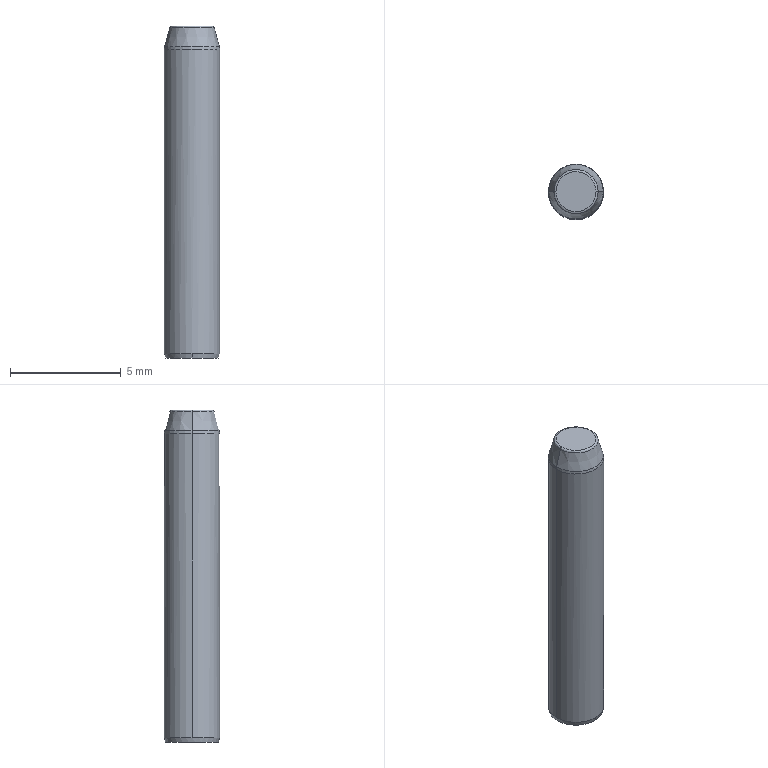Part | SolidWorks | features BaseBody 1 | 1 solid | 12 faces | box 2.5 x 2.5 x 15 mm | volume 72.605 mm3 | spline 4 | cone 4 | cylinder 2 | plane 2 | commonest cylinder face diameters 2.5 x2
STEP:
#1=CARTESIAN_POINT('',(1.233,0.,14.064));
#2=VERTEX_POINT('',#1);
#3=CARTESIAN_POINT('',(-1.233,0.,14.064));
#4=VERTEX_POINT('',#3);
#5=CARTESIAN_POINT('',(0.,0.,14.064));
#6=DIRECTION('',(0.,0.,-1.));
#7=DIRECTION('',(1.,0.,0.));
#8=AXIS2_PLACEMENT_3D('',#5,#6,#7);
#9=CIRCLE('',#8,1.233);
#10=EDGE_CURVE('',#2,#4,#9,.T.);
#11=ORIENTED_EDGE('',*,*,#10,.T.);
#12=CARTESIAN_POINT('',(-1.25,0.,13.934));
#13=VERTEX_POINT('',#12);
#14=CARTESIAN_POINT('',(-0.75,0.,13.934));
#15=DIRECTION('',(0.,-1.,0.));
#16=DIRECTION('',(-1.,0.,0.));
#17=AXIS2_PLACEMENT_3D('',#14,#15,#16);
#18=CIRCLE('',#17,0.5);
#19=EDGE_CURVE('',#4,#13,#18,.T.);
#20=ORIENTED_EDGE('',*,*,#19,.T.);
#21=CARTESIAN_POINT('',(1.25,0.,13.934));
#22=VERTEX_POINT('',#21);
#23=CARTESIAN_POINT('',(0.,0.,13.934));
#24=DIRECTION('',(0.,0.,-1.));
#25=DIRECTION('',(1.,0.,0.));
#26=AXIS2_PLACEMENT_3D('',#23,#24,#25);
#27=CIRCLE('',#26,1.25);
#28=EDGE_CURVE('',#22,#13,#27,.T.);
#29=ORIENTED_EDGE('',*,*,#28,.F.);
#30=CARTESIAN_POINT('',(0.75,0.,13.934));
#31=DIRECTION('',(0.,1.,0.));
#32=DIRECTION('',(1.,0.,0.));
#33=AXIS2_PLACEMENT_3D('',#30,#31,#32);
#34=CIRCLE('',#33,0.5);
#35=EDGE_CURVE('',#2,#22,#34,.T.);
#36=ORIENTED_EDGE('',*,*,#35,.F.);
#37=EDGE_LOOP('',(#11,#20,#29,#36));
#38=FACE_OUTER_BOUND('',#37,.T.);
#39=CARTESIAN_POINT('',(-1.233,0.,14.064));
#40=CARTESIAN_POINT('',(-1.233,-2.466,14.064));
#41=CARTESIAN_POINT('',(1.233,-2.466,14.064));
#42=CARTESIAN_POINT('',(1.233,0.,14.064));
#43=CARTESIAN_POINT('',(-1.244,0.,14.021));
#44=CARTESIAN_POINT('',(-1.244,-2.489,14.021));
#45=CARTESIAN_POINT('',(1.244,-2.489,14.021));
#46=CARTESIAN_POINT('',(1.244,0.,14.021));
#47=CARTESIAN_POINT('',(-1.25,0.,13.978));
#48=CARTESIAN_POINT('',(-1.25,-2.5,13.978));
#49=CARTESIAN_POINT('',(1.25,-2.5,13.978));
#50=CARTESIAN_POINT('',(1.25,0.,13.978));
#51=CARTESIAN_POINT('',(-1.25,0.,13.934));
#52=CARTESIAN_POINT('',(-1.25,-2.5,13.934));
#53=CARTESIAN_POINT('',(1.25,-2.5,13.934));
#54=CARTESIAN_POINT('',(1.25,0.,13.934));
#55=(BOUNDED_SURFACE()B_SPLINE_SURFACE(3,3,((#39,#40,#41,#42),(#43,#44,#45,#46),(#47,#48,#49,#50),(#51,#52,#53,#54)),.UNSPECIFIED.,.F.,.F.,.T.)B_SPLINE_SURFACE_WITH_KNOTS((4,4),(4,4),(0.,1.),(0.,1.),.UNSPECIFIED.)GEOMETRIC_REPRESENTATION_ITEM()RATIONAL_B_SPLINE_SURFACE(((1.,0.3333,0.3333,1.),(0.9943,0.3314,0.3314,0.9943),(0.9943,0.3314,0.3314,0.9943),(1.,0.3333,0.3333,1.)))REPRESENTATION_ITEM('')SURFACE());
#56=ADVANCED_FACE('',(#38),#55,.T.);
#57=CARTESIAN_POINT('',(1.002,0.,14.926));
#58=VERTEX_POINT('',#57);
#59=CARTESIAN_POINT('',(-1.002,0.,14.926));
#60=VERTEX_POINT('',#59);
#61=CARTESIAN_POINT('',(0.,0.,14.926));
#62=DIRECTION('',(0.,0.,-1.));
#63=DIRECTION('',(-1.,0.,0.));
#64=AXIS2_PLACEMENT_3D('',#61,#62,#63);
#65=CIRCLE('',#64,1.002);
#66=EDGE_CURVE('',#58,#60,#65,.T.);
#67=ORIENTED_EDGE('',*,*,#66,.F.);
#68=CARTESIAN_POINT('',(0.9053,0.,15.));
#69=VERTEX_POINT('',#68);
#70=CARTESIAN_POINT('',(0.9053,0.,14.9));
#71=DIRECTION('',(0.,-1.,0.));
#72=DIRECTION('',(1.,0.,0.));
#73=AXIS2_PLACEMENT_3D('',#70,#71,#72);
#74=CIRCLE('',#73,0.1);
#75=EDGE_CURVE('',#58,#69,#74,.T.);
#76=ORIENTED_EDGE('',*,*,#75,.T.);
#77=CARTESIAN_POINT('',(-0.9053,0.,15.));
#78=VERTEX_POINT('',#77);
#79=CARTESIAN_POINT('',(0.9053,0.,15.));
#80=CARTESIAN_POINT('',(0.9053,-1.811,15.));
#81=CARTESIAN_POINT('',(-0.9053,-1.811,15.));
#82=CARTESIAN_POINT('',(-0.9053,0.,15.));
#83=(BOUNDED_CURVE()B_SPLINE_CURVE(3,(#79,#80,#81,#82),.UNSPECIFIED.,.F.,.F.)B_SPLINE_CURVE_WITH_KNOTS((4,4),(0.,0.5),.UNSPECIFIED.)CURVE()GEOMETRIC_REPRESENTATION_ITEM()RATIONAL_B_SPLINE_CURVE((1.,0.3333,0.3333,1.))REPRESENTATION_ITEM(''));
#84=EDGE_CURVE('',#69,#78,#83,.T.);
#85=ORIENTED_EDGE('',*,*,#84,.T.);
#86=CARTESIAN_POINT('',(-0.9053,0.,14.9));
#87=DIRECTION('',(0.,1.,0.));
#88=DIRECTION('',(-1.,0.,0.));
#89=AXIS2_PLACEMENT_3D('',#86,#87,#88);
#90=CIRCLE('',#89,0.1);
#91=EDGE_CURVE('',#60,#78,#90,.T.);
#92=ORIENTED_EDGE('',*,*,#91,.F.);
#93=EDGE_LOOP('',(#67,#76,#85,#92));
#94=FACE_OUTER_BOUND('',#93,.T.);
#95=CARTESIAN_POINT('',(1.002,0.,14.926));
#96=CARTESIAN_POINT('',(1.002,-2.004,14.926));
#97=CARTESIAN_POINT('',(-1.002,-2.004,14.926));
#98=CARTESIAN_POINT('',(-1.002,0.,14.926));
#99=CARTESIAN_POINT('',(0.9897,0.,14.971));
#100=CARTESIAN_POINT('',(0.9897,-1.979,14.971));
#101=CARTESIAN_POINT('',(-0.9897,-1.979,14.971));
#102=CARTESIAN_POINT('',(-0.9897,0.,14.971));
#103=CARTESIAN_POINT('',(0.9524,0.,15.));
#104=CARTESIAN_POINT('',(0.9524,-1.905,15.));
#105=CARTESIAN_POINT('',(-0.9524,-1.905,15.));
#106=CARTESIAN_POINT('',(-0.9524,0.,15.));
#107=CARTESIAN_POINT('',(0.9053,0.,15.));
#108=CARTESIAN_POINT('',(0.9053,-1.811,15.));
#109=CARTESIAN_POINT('',(-0.9053,-1.811,15.));
#110=CARTESIAN_POINT('',(-0.9053,0.,15.));
#111=(BOUNDED_SURFACE()B_SPLINE_SURFACE(3,3,((#95,#96,#97,#98),(#99,#100,#101,#102),(#103,#104,#105,#106),(#107,#108,#109,#110)),.UNSPECIFIED.,.F.,.F.,.T.)B_SPLINE_SURFACE_WITH_KNOTS((4,4),(4,4),(0.,1.),(0.,1.),.UNSPECIFIED.)GEOMETRIC_REPRESENTATION_ITEM()RATIONAL_B_SPLINE_SURFACE(((1.,0.3333,0.3333,1.),(0.8622,0.2874,0.2874,0.8622),(0.8622,0.2874,0.2874,0.8622),(1.,0.3333,0.3333,1.)))REPRESENTATION_ITEM('')SURFACE());
#112=ADVANCED_FACE('',(#94),#111,.T.);
#113=CARTESIAN_POINT('',(0.,1.25,0.2));
#114=VERTEX_POINT('',#113);
#115=CARTESIAN_POINT('',(-1.25,0.,0.2));
#116=VERTEX_POINT('',#115);
#117=CARTESIAN_POINT('',(0.,0.,0.2));
#118=DIRECTION('',(0.,0.,1.));
#119=DIRECTION('',(1.,0.,0.));
#120=AXIS2_PLACEMENT_3D('',#117,#118,#119);
#121=CIRCLE('',#120,1.25);
#122=EDGE_CURVE('',#114,#116,#121,.T.);
#123=ORIENTED_EDGE('',*,*,#122,.T.);
#124=CARTESIAN_POINT('',(-1.25,0.,0.));
#125=DIRECTION('',(0.,0.,1.));
#126=VECTOR('',#125,1000.);
#127=LINE('',#124,#126);
#128=EDGE_CURVE('',#116,#13,#127,.T.);
#129=ORIENTED_EDGE('',*,*,#128,.T.);
#130=CARTESIAN_POINT('',(0.,0.,13.934));
#131=DIRECTION('',(0.,0.,-1.));
#132=DIRECTION('',(1.,0.,0.));
#133=AXIS2_PLACEMENT_3D('',#130,#131,#132);
#134=CIRCLE('',#133,1.25);
#135=EDGE_CURVE('',#13,#22,#134,.T.);
#136=ORIENTED_EDGE('',*,*,#135,.T.);
#137=CARTESIAN_POINT('',(1.25,0.,0.2));
#138=VERTEX_POINT('',#137);
#139=CARTESIAN_POINT('',(1.25,0.,0.));
#140=DIRECTION('',(0.,0.,1.));
#141=VECTOR('',#140,1000.);
#142=LINE('',#139,#141);
#143=EDGE_CURVE('',#138,#22,#142,.T.);
#144=ORIENTED_EDGE('',*,*,#143,.F.);
#145=CARTESIAN_POINT('',(0.,0.,0.2));
#146=DIRECTION('',(0.,0.,1.));
#147=DIRECTION('',(1.,0.,0.));
#148=AXIS2_PLACEMENT_3D('',#145,#146,#147);
#149=CIRCLE('',#148,1.25);
#150=EDGE_CURVE('',#138,#114,#149,.T.);
#151=ORIENTED_EDGE('',*,*,#150,.T.);
#152=EDGE_LOOP('',(#123,#129,#136,#144,#151));
#153=FACE_OUTER_BOUND('',#152,.T.);
#154=CARTESIAN_POINT('',(0.,0.,0.));
#155=DIRECTION('',(0.,0.,1.));
#156=DIRECTION('',(1.,0.,0.));
#157=AXIS2_PLACEMENT_3D('',#154,#155,#156);
#158=CYLINDRICAL_SURFACE('',#157,1.25);
#159=ADVANCED_FACE('',(#153),#158,.T.);
#160=CARTESIAN_POINT('',(0.,-1.196,0.));
#161=VERTEX_POINT('',#160);
#162=CARTESIAN_POINT('',(0.,1.196,0.));
#163=VERTEX_POINT('',#162);
#164=CARTESIAN_POINT('',(0.,0.,0.));
#165=DIRECTION('',(0.,0.,1.));
#166=DIRECTION('',(0.,-1.,0.));
#167=AXIS2_PLACEMENT_3D('',#164,#165,#166);
#168=CIRCLE('',#167,1.196);
#169=EDGE_CURVE('',#161,#163,#168,.T.);
#170=ORIENTED_EDGE('',*,*,#169,.T.);
#171=CARTESIAN_POINT('',(0.,1.25,0.2));
#172=DIRECTION('',(0.,0.2588,0.9659));
#173=VECTOR('',#172,1000.);
#174=LINE('',#171,#173);
#175=EDGE_CURVE('',#163,#114,#174,.T.);
#176=ORIENTED_EDGE('',*,*,#175,.T.);
#177=ORIENTED_EDGE('',*,*,#150,.F.);
#178=CARTESIAN_POINT('',(0.,-1.25,0.2));
#179=VERTEX_POINT('',#178);
#180=CARTESIAN_POINT('',(0.,0.,0.2));
#181=DIRECTION('',(0.,0.,1.));
#182=DIRECTION('',(1.,0.,0.));
#183=AXIS2_PLACEMENT_3D('',#180,#181,#182);
#184=CIRCLE('',#183,1.25);
#185=EDGE_CURVE('',#179,#138,#184,.T.);
#186=ORIENTED_EDGE('',*,*,#185,.F.);
#187=CARTESIAN_POINT('',(0.,-1.25,0.2));
#188=DIRECTION('',(0.,-0.2588,0.9659));
#189=VECTOR('',#188,1000.);
#190=LINE('',#187,#189);
#191=EDGE_CURVE('',#161,#179,#190,.T.);
#192=ORIENTED_EDGE('',*,*,#191,.F.);
#193=EDGE_LOOP('',(#170,#176,#177,#186,#192));
#194=FACE_OUTER_BOUND('',#193,.T.);
#195=CARTESIAN_POINT('',(0.,0.,0.2));
#196=DIRECTION('',(0.,0.,1.));
#197=DIRECTION('',(0.,-1.,0.));
#198=AXIS2_PLACEMENT_3D('',#195,#196,#197);
#199=CONICAL_SURFACE('',#198,1.25,0.2618);
#200=ADVANCED_FACE('',(#194),#199,.T.);
#201=CARTESIAN_POINT('',(0.,0.,14.926));
#202=DIRECTION('',(0.,0.,-1.));
#203=DIRECTION('',(-1.,0.,0.));
#204=AXIS2_PLACEMENT_3D('',#201,#202,#203);
#205=CIRCLE('',#204,1.002);
#206=EDGE_CURVE('',#60,#58,#205,.T.);
#207=ORIENTED_EDGE('',*,*,#206,.T.);
#208=CARTESIAN_POINT('',(1.233,0.,14.064));
#209=DIRECTION('',(0.2588,0.,-0.9659));
#210=VECTOR('',#209,1000.);
#211=LINE('',#208,#210);
#212=EDGE_CURVE('',#58,#2,#211,.T.);
#213=ORIENTED_EDGE('',*,*,#212,.T.);
#214=CARTESIAN_POINT('',(0.,0.,14.064));
#215=DIRECTION('',(0.,0.,-1.));
#216=DIRECTION('',(1.,0.,0.));
#217=AXIS2_PLACEMENT_3D('',#214,#215,#216);
#218=CIRCLE('',#217,1.233);
#219=EDGE_CURVE('',#4,#2,#218,.T.);
#220=ORIENTED_EDGE('',*,*,#219,.F.);
#221=CARTESIAN_POINT('',(-1.233,0.,14.064));
#222=DIRECTION('',(-0.2588,0.,-0.9659));
#223=VECTOR('',#222,1000.);
#224=LINE('',#221,#223);
#225=EDGE_CURVE('',#60,#4,#224,.T.);
#226=ORIENTED_EDGE('',*,*,#225,.F.);
#227=EDGE_LOOP('',(#207,#213,#220,#226));
#228=FACE_OUTER_BOUND('',#227,.T.);
#229=CARTESIAN_POINT('',(0.,0.,14.064));
#230=DIRECTION('',(0.,0.,-1.));
#231=DIRECTION('',(-1.,0.,0.));
#232=AXIS2_PLACEMENT_3D('',#229,#230,#231);
#233=CONICAL_SURFACE('',#232,1.233,0.2618);
#234=ADVANCED_FACE('',(#228),#233,.T.);
#235=ORIENTED_EDGE('',*,*,#128,.F.);
#236=CARTESIAN_POINT('',(0.,0.,0.2));
#237=DIRECTION('',(0.,0.,1.));
#238=DIRECTION('',(1.,0.,0.));
#239=AXIS2_PLACEMENT_3D('',#236,#237,#238);
#240=CIRCLE('',#239,1.25);
#241=EDGE_CURVE('',#116,#179,#240,.T.);
#242=ORIENTED_EDGE('',*,*,#241,.T.);
#243=ORIENTED_EDGE('',*,*,#185,.T.);
#244=ORIENTED_EDGE('',*,*,#143,.T.);
#245=ORIENTED_EDGE('',*,*,#28,.T.);
#246=EDGE_LOOP('',(#235,#242,#243,#244,#245));
#247=FACE_OUTER_BOUND('',#246,.T.);
#248=CARTESIAN_POINT('',(0.,0.,0.));
#249=DIRECTION('',(0.,0.,1.));
#250=DIRECTION('',(1.,0.,0.));
#251=AXIS2_PLACEMENT_3D('',#248,#249,#250);
#252=CYLINDRICAL_SURFACE('',#251,1.25);
#253=ADVANCED_FACE('',(#247),#252,.T.);
#254=ORIENTED_EDGE('',*,*,#19,.F.);
#255=ORIENTED_EDGE('',*,*,#219,.T.);
#256=ORIENTED_EDGE('',*,*,#35,.T.);
#257=ORIENTED_EDGE('',*,*,#135,.F.);
#258=EDGE_LOOP('',(#254,#255,#256,#257));
#259=FACE_OUTER_BOUND('',#258,.T.);
#260=CARTESIAN_POINT('',(1.233,0.,14.064));
#261=CARTESIAN_POINT('',(1.233,2.466,14.064));
#262=CARTESIAN_POINT('',(-1.233,2.466,14.064));
#263=CARTESIAN_POINT('',(-1.233,0.,14.064));
#264=CARTESIAN_POINT('',(1.244,0.,14.021));
#265=CARTESIAN_POINT('',(1.244,2.489,14.021));
#266=CARTESIAN_POINT('',(-1.244,2.489,14.021));
#267=CARTESIAN_POINT('',(-1.244,0.,14.021));
#268=CARTESIAN_POINT('',(1.25,0.,13.978));
#269=CARTESIAN_POINT('',(1.25,2.5,13.978));
#270=CARTESIAN_POINT('',(-1.25,2.5,13.978));
#271=CARTESIAN_POINT('',(-1.25,0.,13.978));
#272=CARTESIAN_POINT('',(1.25,0.,13.934));
#273=CARTESIAN_POINT('',(1.25,2.5,13.934));
#274=CARTESIAN_POINT('',(-1.25,2.5,13.934));
#275=CARTESIAN_POINT('',(-1.25,0.,13.934));
#276=(BOUNDED_SURFACE()B_SPLINE_SURFACE(3,3,((#260,#261,#262,#263),(#264,#265,#266,#267),(#268,#269,#270,#271),(#272,#273,#274,#275)),.UNSPECIFIED.,.F.,.F.,.F.)B_SPLINE_SURFACE_WITH_KNOTS((4,4),(4,4),(0.,1.),(0.,1.),.UNSPECIFIED.)GEOMETRIC_REPRESENTATION_ITEM()RATIONAL_B_SPLINE_SURFACE(((1.,0.3333,0.3333,1.),(0.9943,0.3314,0.3314,0.9943),(0.9943,0.3314,0.3314,0.9943),(1.,0.3333,0.3333,1.)))REPRESENTATION_ITEM('')SURFACE());
#277=ADVANCED_FACE('',(#259),#276,.T.);
#278=ORIENTED_EDGE('',*,*,#175,.F.);
#279=CARTESIAN_POINT('',(0.,0.,0.));
#280=DIRECTION('',(0.,0.,1.));
#281=DIRECTION('',(0.,-1.,0.));
#282=AXIS2_PLACEMENT_3D('',#279,#280,#281);
#283=CIRCLE('',#282,1.196);
#284=EDGE_CURVE('',#163,#161,#283,.T.);
#285=ORIENTED_EDGE('',*,*,#284,.T.);
#286=ORIENTED_EDGE('',*,*,#191,.T.);
#287=ORIENTED_EDGE('',*,*,#241,.F.);
#288=ORIENTED_EDGE('',*,*,#122,.F.);
#289=EDGE_LOOP('',(#278,#285,#286,#287,#288));
#290=FACE_OUTER_BOUND('',#289,.T.);
#291=CARTESIAN_POINT('',(0.,0.,0.2));
#292=DIRECTION('',(0.,0.,1.));
#293=DIRECTION('',(0.,-1.,0.));
#294=AXIS2_PLACEMENT_3D('',#291,#292,#293);
#295=CONICAL_SURFACE('',#294,1.25,0.2618);
#296=ADVANCED_FACE('',(#290),#295,.T.);
#297=ORIENTED_EDGE('',*,*,#212,.F.);
#298=ORIENTED_EDGE('',*,*,#66,.T.);
#299=ORIENTED_EDGE('',*,*,#225,.T.);
#300=ORIENTED_EDGE('',*,*,#10,.F.);
#301=EDGE_LOOP('',(#297,#298,#299,#300));
#302=FACE_OUTER_BOUND('',#301,.T.);
#303=CARTESIAN_POINT('',(0.,0.,14.064));
#304=DIRECTION('',(0.,0.,-1.));
#305=DIRECTION('',(-1.,0.,0.));
#306=AXIS2_PLACEMENT_3D('',#303,#304,#305);
#307=CONICAL_SURFACE('',#306,1.233,0.2618);
#308=ADVANCED_FACE('',(#302),#307,.T.);
#309=ORIENTED_EDGE('',*,*,#169,.F.);
#310=ORIENTED_EDGE('',*,*,#284,.F.);
#311=EDGE_LOOP('',(#309,#310));
#312=FACE_OUTER_BOUND('',#311,.T.);
#313=CARTESIAN_POINT('',(0.,0.,0.));
#314=DIRECTION('',(0.,0.,-1.));
#315=DIRECTION('',(-1.,0.,0.));
#316=AXIS2_PLACEMENT_3D('',#313,#314,#315);
#317=PLANE('',#316);
#318=ADVANCED_FACE('',(#312),#317,.T.);
#319=ORIENTED_EDGE('',*,*,#75,.F.);
#320=ORIENTED_EDGE('',*,*,#206,.F.);
#321=ORIENTED_EDGE('',*,*,#91,.T.);
#322=CARTESIAN_POINT('',(-0.9053,0.,15.));
#323=CARTESIAN_POINT('',(-0.9053,1.811,15.));
#324=CARTESIAN_POINT('',(0.9053,1.811,15.));
#325=CARTESIAN_POINT('',(0.9053,0.,15.));
#326=(BOUNDED_CURVE()B_SPLINE_CURVE(3,(#322,#323,#324,#325),.UNSPECIFIED.,.F.,.F.)B_SPLINE_CURVE_WITH_KNOTS((4,4),(0.5,1.),.UNSPECIFIED.)CURVE()GEOMETRIC_REPRESENTATION_ITEM()RATIONAL_B_SPLINE_CURVE((1.,0.3333,0.3333,1.))REPRESENTATION_ITEM(''));
#327=EDGE_CURVE('',#78,#69,#326,.T.);
#328=ORIENTED_EDGE('',*,*,#327,.T.);
#329=EDGE_LOOP('',(#319,#320,#321,#328));
#330=FACE_OUTER_BOUND('',#329,.T.);
#331=CARTESIAN_POINT('',(-1.002,0.,14.926));
#332=CARTESIAN_POINT('',(-1.002,2.004,14.926));
#333=CARTESIAN_POINT('',(1.002,2.004,14.926));
#334=CARTESIAN_POINT('',(1.002,0.,14.926));
#335=CARTESIAN_POINT('',(-0.9897,0.,14.971));
#336=CARTESIAN_POINT('',(-0.9897,1.979,14.971));
#337=CARTESIAN_POINT('',(0.9897,1.979,14.971));
#338=CARTESIAN_POINT('',(0.9897,0.,14.971));
#339=CARTESIAN_POINT('',(-0.9524,0.,15.));
#340=CARTESIAN_POINT('',(-0.9524,1.905,15.));
#341=CARTESIAN_POINT('',(0.9524,1.905,15.));
#342=CARTESIAN_POINT('',(0.9524,0.,15.));
#343=CARTESIAN_POINT('',(-0.9053,0.,15.));
#344=CARTESIAN_POINT('',(-0.9053,1.811,15.));
#345=CARTESIAN_POINT('',(0.9053,1.811,15.));
#346=CARTESIAN_POINT('',(0.9053,0.,15.));
#347=(BOUNDED_SURFACE()B_SPLINE_SURFACE(3,3,((#331,#332,#333,#334),(#335,#336,#337,#338),(#339,#340,#341,#342),(#343,#344,#345,#346)),.UNSPECIFIED.,.F.,.F.,.T.)B_SPLINE_SURFACE_WITH_KNOTS((4,4),(4,4),(0.,1.),(0.,1.),.UNSPECIFIED.)GEOMETRIC_REPRESENTATION_ITEM()RATIONAL_B_SPLINE_SURFACE(((1.,0.3333,0.3333,1.),(0.8622,0.2874,0.2874,0.8622),(0.8622,0.2874,0.2874,0.8622),(1.,0.3333,0.3333,1.)))REPRESENTATION_ITEM('')SURFACE());
#348=ADVANCED_FACE('',(#330),#347,.T.);
#349=ORIENTED_EDGE('',*,*,#327,.F.);
#350=ORIENTED_EDGE('',*,*,#84,.F.);
#351=EDGE_LOOP('',(#349,#350));
#352=FACE_OUTER_BOUND('',#351,.T.);
#353=CARTESIAN_POINT('',(0.,0.,15.));
#354=DIRECTION('',(0.,0.,-1.));
#355=DIRECTION('',(-1.,0.,0.));
#356=AXIS2_PLACEMENT_3D('',#353,#354,#355);
#357=PLANE('',#356);
#358=ADVANCED_FACE('',(#352),#357,.F.);
#359=CLOSED_SHELL('',(#56,#112,#159,#200,#234,#253,#277,#296,#308,#318,#348,#358));
#360=MANIFOLD_SOLID_BREP('',#359);
#361=CARTESIAN_POINT('',(0.,0.,0.));
#362=DIRECTION('',(0.,0.,1.));
#363=DIRECTION('',(1.,0.,0.));
#364=AXIS2_PLACEMENT_3D('',#361,#362,#363);
#365=(LENGTH_UNIT()NAMED_UNIT(*)SI_UNIT(.MILLI.,.METRE.));
#366=UNCERTAINTY_MEASURE_WITH_UNIT(LENGTH_MEASURE(0.00001),#365,'','');
#367=(NAMED_UNIT(*)PLANE_ANGLE_UNIT()SI_UNIT($,.RADIAN.));
#368=(NAMED_UNIT(*)SI_UNIT($,.STERADIAN.)SOLID_ANGLE_UNIT());
#369=(GEOMETRIC_REPRESENTATION_CONTEXT(3)GLOBAL_UNCERTAINTY_ASSIGNED_CONTEXT((#366))GLOBAL_UNIT_ASSIGNED_CONTEXT((#365,#367,#368))REPRESENTATION_CONTEXT('',''));
#370=ADVANCED_BREP_SHAPE_REPRESENTATION('',(#360,#364),#369);